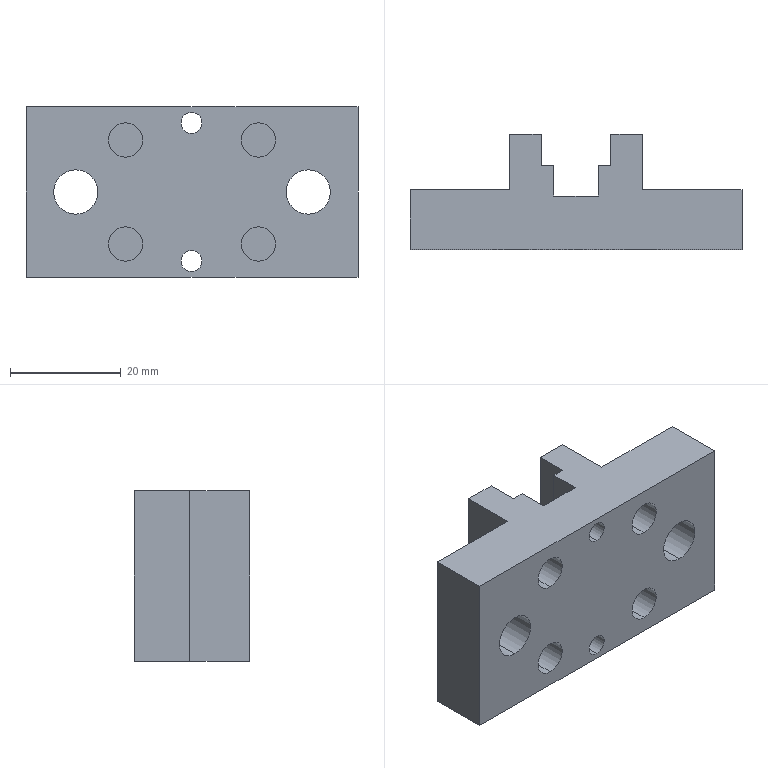Part | STEP file | Riveting floating block | 1 solid | 38 faces | box 60 x 20.8 x 30.8 mm | volume 21870 mm3 | plane 22 | cylinder 16 | commonest cylinder face diameters 6.2 x8 3.8 x4 8 x4